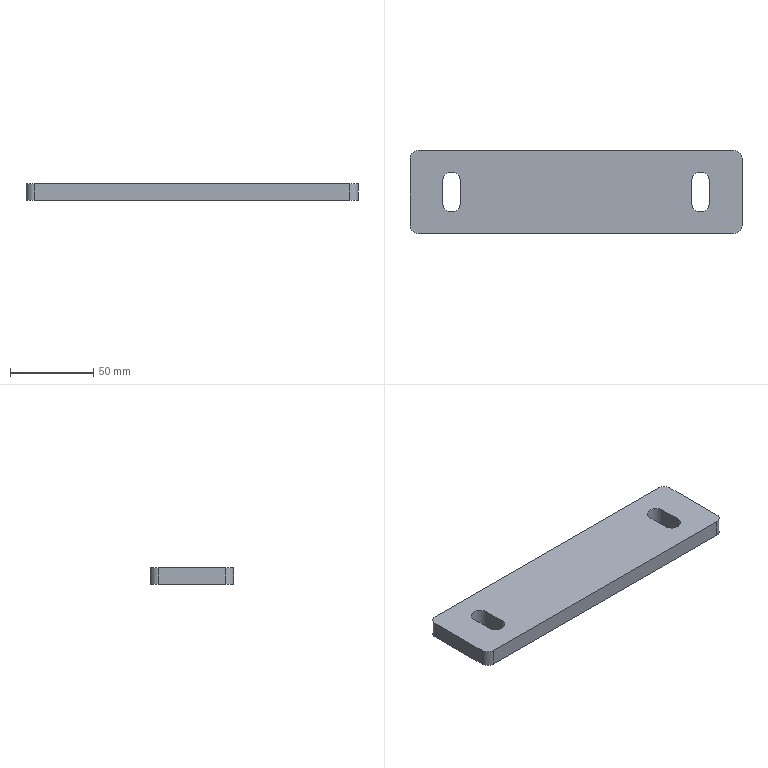Part | STEP file | 1 solid | 18 faces | box 200 x 50 x 10 mm | volume 95025 mm3 | plane 10 | cylinder 8 | commonest cylinder face diameters 10 x4 11 x4
STEP:
#1=CARTESIAN_POINT('',(0.,0.,0.));
#2=DIRECTION('',(0.,0.,1.));
#3=DIRECTION('',(1.,0.,0.));
#4=AXIS2_PLACEMENT_3D('',#1,#2,#3);
#5=CARTESIAN_POINT('',(-80.5,6.5,10.));
#6=VERTEX_POINT('',#5);
#7=CARTESIAN_POINT('',(-69.5,6.5,10.));
#8=VERTEX_POINT('',#7);
#9=CARTESIAN_POINT('',(-75.,6.5,10.));
#10=DIRECTION('',(0.,0.,-1.));
#11=DIRECTION('',(1.,0.,0.));
#12=AXIS2_PLACEMENT_3D('',#9,#10,#11);
#13=CIRCLE('',#12,5.5);
#14=CARTESIAN_POINT('',(95.,20.,10.));
#15=DIRECTION('',(0.,0.,1.));
#16=DIRECTION('',(1.,0.,0.));
#17=AXIS2_PLACEMENT_3D('',#14,#15,#16);
#18=PLANE('',#17);
#19=CARTESIAN_POINT('',(-164.5,-13.5));
#20=CARTESIAN_POINT('',(-164.5,-23.026));
#21=CARTESIAN_POINT('',(-172.75,-18.263));
#22=CARTESIAN_POINT('',(-181.,-13.5));
#23=CARTESIAN_POINT('',(-172.75,-8.737));
#24=CARTESIAN_POINT('',(-164.5,-3.974));
#25=CARTESIAN_POINT('',(-164.5,-13.5));
#26=(BOUNDED_CURVE()B_SPLINE_CURVE(2,(#19,#20,#21,#22,#23,#24,#25),.UNSPECIFIED.,.T.,.F.)B_SPLINE_CURVE_WITH_KNOTS((1,2,2,2,2,1),(-2.094,0.,2.094,4.189,6.283,8.378),.UNSPECIFIED.)CURVE()GEOMETRIC_REPRESENTATION_ITEM()RATIONAL_B_SPLINE_CURVE((1.,0.5,1.,0.5,1.,0.5,1.))REPRESENTATION_ITEM(''));
#27=(GEOMETRIC_REPRESENTATION_CONTEXT(2)PARAMETRIC_REPRESENTATION_CONTEXT()REPRESENTATION_CONTEXT('',''));
#28=DEFINITIONAL_REPRESENTATION('',(#26),#27);
#29=PCURVE('',#18,#28);
#30=CARTESIAN_POINT('',(-75.,6.5,0.));
#31=DIRECTION('',(0.,0.,1.));
#32=DIRECTION('',(1.,0.,0.));
#33=AXIS2_PLACEMENT_3D('',#30,#31,#32);
#34=CYLINDRICAL_SURFACE('',#33,5.5);
#35=CARTESIAN_POINT('',(6.283,10.));
#36=DIRECTION('',(-1.,0.));
#37=VECTOR('',#36,1.);
#38=LINE('',#35,#37);
#39=(GEOMETRIC_REPRESENTATION_CONTEXT(2)PARAMETRIC_REPRESENTATION_CONTEXT()REPRESENTATION_CONTEXT('',''));
#40=DEFINITIONAL_REPRESENTATION('',(#38),#39);
#41=PCURVE('',#34,#40);
#42=SURFACE_CURVE('',#13,(#29,#41),.PCURVE_S1.);
#43=EDGE_CURVE('',#6,#8,#42,.T.);
#44=ORIENTED_EDGE('',*,*,#43,.T.);
#45=CARTESIAN_POINT('',(-69.5,-6.5,10.));
#46=VERTEX_POINT('',#45);
#47=CARTESIAN_POINT('',(-69.5,-6.5,10.));
#48=DIRECTION('',(0.,-1.,0.));
#49=VECTOR('',#48,1.);
#50=LINE('',#47,#49);
#51=CARTESIAN_POINT('',(-164.5,-26.5));
#52=DIRECTION('',(0.,-1.));
#53=VECTOR('',#52,1.);
#54=LINE('',#51,#53);
#55=(GEOMETRIC_REPRESENTATION_CONTEXT(2)PARAMETRIC_REPRESENTATION_CONTEXT()REPRESENTATION_CONTEXT('',''));
#56=DEFINITIONAL_REPRESENTATION('',(#54),#55);
#57=PCURVE('',#18,#56);
#58=CARTESIAN_POINT('',(-69.5,-6.5,0.));
#59=DIRECTION('',(1.,0.,0.));
#60=DIRECTION('',(0.,1.,0.));
#61=AXIS2_PLACEMENT_3D('',#58,#59,#60);
#62=PLANE('',#61);
#63=CARTESIAN_POINT('',(0.,10.));
#64=DIRECTION('',(-1.,0.));
#65=VECTOR('',#64,1.);
#66=LINE('',#63,#65);
#67=(GEOMETRIC_REPRESENTATION_CONTEXT(2)PARAMETRIC_REPRESENTATION_CONTEXT()REPRESENTATION_CONTEXT('',''));
#68=DEFINITIONAL_REPRESENTATION('',(#66),#67);
#69=PCURVE('',#62,#68);
#70=SURFACE_CURVE('',#50,(#57,#69),.PCURVE_S1.);
#71=EDGE_CURVE('',#8,#46,#70,.T.);
#72=ORIENTED_EDGE('',*,*,#71,.T.);
#73=CARTESIAN_POINT('',(-80.5,-6.5,10.));
#74=VERTEX_POINT('',#73);
#75=CARTESIAN_POINT('',(-75.,-6.5,10.));
#76=DIRECTION('',(0.,0.,-1.));
#77=DIRECTION('',(1.,0.,0.));
#78=AXIS2_PLACEMENT_3D('',#75,#76,#77);
#79=CIRCLE('',#78,5.5);
#80=CARTESIAN_POINT('',(-164.5,-26.5));
#81=CARTESIAN_POINT('',(-164.5,-36.026));
#82=CARTESIAN_POINT('',(-172.75,-31.263));
#83=CARTESIAN_POINT('',(-181.,-26.5));
#84=CARTESIAN_POINT('',(-172.75,-21.737));
#85=CARTESIAN_POINT('',(-164.5,-16.974));
#86=CARTESIAN_POINT('',(-164.5,-26.5));
#87=(BOUNDED_CURVE()B_SPLINE_CURVE(2,(#80,#81,#82,#83,#84,#85,#86),.UNSPECIFIED.,.T.,.F.)B_SPLINE_CURVE_WITH_KNOTS((1,2,2,2,2,1),(-2.094,0.,2.094,4.189,6.283,8.378),.UNSPECIFIED.)CURVE()GEOMETRIC_REPRESENTATION_ITEM()RATIONAL_B_SPLINE_CURVE((1.,0.5,1.,0.5,1.,0.5,1.))REPRESENTATION_ITEM(''));
#88=(GEOMETRIC_REPRESENTATION_CONTEXT(2)PARAMETRIC_REPRESENTATION_CONTEXT()REPRESENTATION_CONTEXT('',''));
#89=DEFINITIONAL_REPRESENTATION('',(#87),#88);
#90=PCURVE('',#18,#89);
#91=CARTESIAN_POINT('',(-75.,-6.5,0.));
#92=DIRECTION('',(0.,0.,1.));
#93=DIRECTION('',(1.,0.,0.));
#94=AXIS2_PLACEMENT_3D('',#91,#92,#93);
#95=CYLINDRICAL_SURFACE('',#94,5.5);
#96=CARTESIAN_POINT('',(6.283,10.));
#97=DIRECTION('',(-1.,0.));
#98=VECTOR('',#97,1.);
#99=LINE('',#96,#98);
#100=(GEOMETRIC_REPRESENTATION_CONTEXT(2)PARAMETRIC_REPRESENTATION_CONTEXT()REPRESENTATION_CONTEXT('',''));
#101=DEFINITIONAL_REPRESENTATION('',(#99),#100);
#102=PCURVE('',#95,#101);
#103=SURFACE_CURVE('',#79,(#90,#102),.PCURVE_S1.);
#104=EDGE_CURVE('',#46,#74,#103,.T.);
#105=ORIENTED_EDGE('',*,*,#104,.T.);
#106=CARTESIAN_POINT('',(-80.5,-6.5,10.));
#107=DIRECTION('',(0.,1.,0.));
#108=VECTOR('',#107,1.);
#109=LINE('',#106,#108);
#110=CARTESIAN_POINT('',(-175.5,-26.5));
#111=DIRECTION('',(0.,1.));
#112=VECTOR('',#111,1.);
#113=LINE('',#110,#112);
#114=(GEOMETRIC_REPRESENTATION_CONTEXT(2)PARAMETRIC_REPRESENTATION_CONTEXT()REPRESENTATION_CONTEXT('',''));
#115=DEFINITIONAL_REPRESENTATION('',(#113),#114);
#116=PCURVE('',#18,#115);
#117=CARTESIAN_POINT('',(-80.5,-6.5,0.));
#118=DIRECTION('',(-1.,0.,0.));
#119=DIRECTION('',(0.,0.,1.));
#120=AXIS2_PLACEMENT_3D('',#117,#118,#119);
#121=PLANE('',#120);
#122=CARTESIAN_POINT('',(10.,0.));
#123=DIRECTION('',(0.,1.));
#124=VECTOR('',#123,1.);
#125=LINE('',#122,#124);
#126=(GEOMETRIC_REPRESENTATION_CONTEXT(2)PARAMETRIC_REPRESENTATION_CONTEXT()REPRESENTATION_CONTEXT('',''));
#127=DEFINITIONAL_REPRESENTATION('',(#125),#126);
#128=PCURVE('',#121,#127);
#129=SURFACE_CURVE('',#109,(#116,#128),.PCURVE_S1.);
#130=EDGE_CURVE('',#74,#6,#129,.T.);
#131=ORIENTED_EDGE('',*,*,#130,.T.);
#132=EDGE_LOOP('',(#44,#72,#105,#131));
#133=FACE_BOUND('',#132,.T.);
#134=CARTESIAN_POINT('',(69.5,6.5,10.));
#135=VERTEX_POINT('',#134);
#136=CARTESIAN_POINT('',(69.5,-6.5,10.));
#137=VERTEX_POINT('',#136);
#138=CARTESIAN_POINT('',(69.5,-6.5,10.));
#139=DIRECTION('',(0.,-1.,0.));
#140=VECTOR('',#139,1.);
#141=LINE('',#138,#140);
#142=CARTESIAN_POINT('',(-25.5,-26.5));
#143=DIRECTION('',(0.,-1.));
#144=VECTOR('',#143,1.);
#145=LINE('',#142,#144);
#146=(GEOMETRIC_REPRESENTATION_CONTEXT(2)PARAMETRIC_REPRESENTATION_CONTEXT()REPRESENTATION_CONTEXT('',''));
#147=DEFINITIONAL_REPRESENTATION('',(#145),#146);
#148=PCURVE('',#18,#147);
#149=CARTESIAN_POINT('',(69.5,-6.5,0.));
#150=DIRECTION('',(1.,0.,0.));
#151=DIRECTION('',(0.,1.,0.));
#152=AXIS2_PLACEMENT_3D('',#149,#150,#151);
#153=PLANE('',#152);
#154=CARTESIAN_POINT('',(0.,10.));
#155=DIRECTION('',(-1.,0.));
#156=VECTOR('',#155,1.);
#157=LINE('',#154,#156);
#158=(GEOMETRIC_REPRESENTATION_CONTEXT(2)PARAMETRIC_REPRESENTATION_CONTEXT()REPRESENTATION_CONTEXT('',''));
#159=DEFINITIONAL_REPRESENTATION('',(#157),#158);
#160=PCURVE('',#153,#159);
#161=SURFACE_CURVE('',#141,(#148,#160),.PCURVE_S1.);
#162=EDGE_CURVE('',#135,#137,#161,.T.);
#163=ORIENTED_EDGE('',*,*,#162,.F.);
#164=CARTESIAN_POINT('',(80.5,6.5,10.));
#165=VERTEX_POINT('',#164);
#166=CARTESIAN_POINT('',(75.,6.5,10.));
#167=DIRECTION('',(0.,0.,-1.));
#168=DIRECTION('',(1.,0.,0.));
#169=AXIS2_PLACEMENT_3D('',#166,#167,#168);
#170=CIRCLE('',#169,5.5);
#171=CARTESIAN_POINT('',(-14.5,-13.5));
#172=CARTESIAN_POINT('',(-14.5,-23.026));
#173=CARTESIAN_POINT('',(-22.75,-18.263));
#174=CARTESIAN_POINT('',(-31.,-13.5));
#175=CARTESIAN_POINT('',(-22.75,-8.737));
#176=CARTESIAN_POINT('',(-14.5,-3.974));
#177=CARTESIAN_POINT('',(-14.5,-13.5));
#178=(BOUNDED_CURVE()B_SPLINE_CURVE(2,(#171,#172,#173,#174,#175,#176,#177),.UNSPECIFIED.,.T.,.F.)B_SPLINE_CURVE_WITH_KNOTS((1,2,2,2,2,1),(-2.094,0.,2.094,4.189,6.283,8.378),.UNSPECIFIED.)CURVE()GEOMETRIC_REPRESENTATION_ITEM()RATIONAL_B_SPLINE_CURVE((1.,0.5,1.,0.5,1.,0.5,1.))REPRESENTATION_ITEM(''));
#179=(GEOMETRIC_REPRESENTATION_CONTEXT(2)PARAMETRIC_REPRESENTATION_CONTEXT()REPRESENTATION_CONTEXT('',''));
#180=DEFINITIONAL_REPRESENTATION('',(#178),#179);
#181=PCURVE('',#18,#180);
#182=CARTESIAN_POINT('',(75.,6.5,0.));
#183=DIRECTION('',(0.,0.,1.));
#184=DIRECTION('',(1.,0.,0.));
#185=AXIS2_PLACEMENT_3D('',#182,#183,#184);
#186=CYLINDRICAL_SURFACE('',#185,5.5);
#187=CARTESIAN_POINT('',(6.283,10.));
#188=DIRECTION('',(-1.,0.));
#189=VECTOR('',#188,1.);
#190=LINE('',#187,#189);
#191=(GEOMETRIC_REPRESENTATION_CONTEXT(2)PARAMETRIC_REPRESENTATION_CONTEXT()REPRESENTATION_CONTEXT('',''));
#192=DEFINITIONAL_REPRESENTATION('',(#190),#191);
#193=PCURVE('',#186,#192);
#194=SURFACE_CURVE('',#170,(#181,#193),.PCURVE_S1.);
#195=EDGE_CURVE('',#135,#165,#194,.T.);
#196=ORIENTED_EDGE('',*,*,#195,.T.);
#197=CARTESIAN_POINT('',(80.5,-6.5,10.));
#198=VERTEX_POINT('',#197);
#199=CARTESIAN_POINT('',(80.5,-6.5,10.));
#200=DIRECTION('',(0.,1.,0.));
#201=VECTOR('',#200,1.);
#202=LINE('',#199,#201);
#203=CARTESIAN_POINT('',(-14.5,-26.5));
#204=DIRECTION('',(0.,1.));
#205=VECTOR('',#204,1.);
#206=LINE('',#203,#205);
#207=(GEOMETRIC_REPRESENTATION_CONTEXT(2)PARAMETRIC_REPRESENTATION_CONTEXT()REPRESENTATION_CONTEXT('',''));
#208=DEFINITIONAL_REPRESENTATION('',(#206),#207);
#209=PCURVE('',#18,#208);
#210=CARTESIAN_POINT('',(80.5,-6.5,0.));
#211=DIRECTION('',(-1.,0.,0.));
#212=DIRECTION('',(0.,0.,1.));
#213=AXIS2_PLACEMENT_3D('',#210,#211,#212);
#214=PLANE('',#213);
#215=CARTESIAN_POINT('',(10.,0.));
#216=DIRECTION('',(0.,1.));
#217=VECTOR('',#216,1.);
#218=LINE('',#215,#217);
#219=(GEOMETRIC_REPRESENTATION_CONTEXT(2)PARAMETRIC_REPRESENTATION_CONTEXT()REPRESENTATION_CONTEXT('',''));
#220=DEFINITIONAL_REPRESENTATION('',(#218),#219);
#221=PCURVE('',#214,#220);
#222=SURFACE_CURVE('',#202,(#209,#221),.PCURVE_S1.);
#223=EDGE_CURVE('',#198,#165,#222,.T.);
#224=ORIENTED_EDGE('',*,*,#223,.F.);
#225=CARTESIAN_POINT('',(75.,-6.5,10.));
#226=DIRECTION('',(0.,0.,-1.));
#227=DIRECTION('',(1.,0.,0.));
#228=AXIS2_PLACEMENT_3D('',#225,#226,#227);
#229=CIRCLE('',#228,5.5);
#230=CARTESIAN_POINT('',(-14.5,-26.5));
#231=CARTESIAN_POINT('',(-14.5,-36.026));
#232=CARTESIAN_POINT('',(-22.75,-31.263));
#233=CARTESIAN_POINT('',(-31.,-26.5));
#234=CARTESIAN_POINT('',(-22.75,-21.737));
#235=CARTESIAN_POINT('',(-14.5,-16.974));
#236=CARTESIAN_POINT('',(-14.5,-26.5));
#237=(BOUNDED_CURVE()B_SPLINE_CURVE(2,(#230,#231,#232,#233,#234,#235,#236),.UNSPECIFIED.,.T.,.F.)B_SPLINE_CURVE_WITH_KNOTS((1,2,2,2,2,1),(-2.094,0.,2.094,4.189,6.283,8.378),.UNSPECIFIED.)CURVE()GEOMETRIC_REPRESENTATION_ITEM()RATIONAL_B_SPLINE_CURVE((1.,0.5,1.,0.5,1.,0.5,1.))REPRESENTATION_ITEM(''));
#238=(GEOMETRIC_REPRESENTATION_CONTEXT(2)PARAMETRIC_REPRESENTATION_CONTEXT()REPRESENTATION_CONTEXT('',''));
#239=DEFINITIONAL_REPRESENTATION('',(#237),#238);
#240=PCURVE('',#18,#239);
#241=CARTESIAN_POINT('',(75.,-6.5,0.));
#242=DIRECTION('',(0.,0.,1.));
#243=DIRECTION('',(1.,0.,0.));
#244=AXIS2_PLACEMENT_3D('',#241,#242,#243);
#245=CYLINDRICAL_SURFACE('',#244,5.5);
#246=CARTESIAN_POINT('',(6.283,10.));
#247=DIRECTION('',(-1.,0.));
#248=VECTOR('',#247,1.);
#249=LINE('',#246,#248);
#250=(GEOMETRIC_REPRESENTATION_CONTEXT(2)PARAMETRIC_REPRESENTATION_CONTEXT()REPRESENTATION_CONTEXT('',''));
#251=DEFINITIONAL_REPRESENTATION('',(#249),#250);
#252=PCURVE('',#245,#251);
#253=SURFACE_CURVE('',#229,(#240,#252),.PCURVE_S1.);
#254=EDGE_CURVE('',#198,#137,#253,.T.);
#255=ORIENTED_EDGE('',*,*,#254,.T.);
#256=EDGE_LOOP('',(#163,#196,#224,#255));
#257=FACE_BOUND('',#256,.T.);
#258=CARTESIAN_POINT('',(100.,-20.,10.));
#259=VERTEX_POINT('',#258);
#260=CARTESIAN_POINT('',(95.,-25.,10.));
#261=VERTEX_POINT('',#260);
#262=CARTESIAN_POINT('',(95.,-20.,10.));
#263=DIRECTION('',(0.,0.,-1.));
#264=DIRECTION('',(-1.,0.,0.));
#265=AXIS2_PLACEMENT_3D('',#262,#263,#264);
#266=CIRCLE('',#265,5.);
#267=CARTESIAN_POINT('',(-5.,-40.));
#268=CARTESIAN_POINT('',(-5.,-31.34));
#269=CARTESIAN_POINT('',(2.5,-35.67));
#270=CARTESIAN_POINT('',(10.,-40.));
#271=CARTESIAN_POINT('',(2.5,-44.33));
#272=CARTESIAN_POINT('',(-5.,-48.66));
#273=CARTESIAN_POINT('',(-5.,-40.));
#274=(BOUNDED_CURVE()B_SPLINE_CURVE(2,(#267,#268,#269,#270,#271,#272,#273),.UNSPECIFIED.,.T.,.F.)B_SPLINE_CURVE_WITH_KNOTS((1,2,2,2,2,1),(-2.094,0.,2.094,4.189,6.283,8.378),.UNSPECIFIED.)CURVE()GEOMETRIC_REPRESENTATION_ITEM()RATIONAL_B_SPLINE_CURVE((1.,0.5,1.,0.5,1.,0.5,1.))REPRESENTATION_ITEM(''));
#275=(GEOMETRIC_REPRESENTATION_CONTEXT(2)PARAMETRIC_REPRESENTATION_CONTEXT()REPRESENTATION_CONTEXT('',''));
#276=DEFINITIONAL_REPRESENTATION('',(#274),#275);
#277=PCURVE('',#18,#276);
#278=CARTESIAN_POINT('',(95.,-20.,10.));
#279=DIRECTION('',(0.,0.,-1.));
#280=DIRECTION('',(-1.,0.,0.));
#281=AXIS2_PLACEMENT_3D('',#278,#279,#280);
#282=CYLINDRICAL_SURFACE('',#281,5.);
#283=CARTESIAN_POINT('',(0.,0.));
#284=DIRECTION('',(1.,0.));
#285=VECTOR('',#284,1.);
#286=LINE('',#283,#285);
#287=(GEOMETRIC_REPRESENTATION_CONTEXT(2)PARAMETRIC_REPRESENTATION_CONTEXT()REPRESENTATION_CONTEXT('',''));
#288=DEFINITIONAL_REPRESENTATION('',(#286),#287);
#289=PCURVE('',#282,#288);
#290=SURFACE_CURVE('',#266,(#277,#289),.PCURVE_S1.);
#291=EDGE_CURVE('',#259,#261,#290,.T.);
#292=ORIENTED_EDGE('',*,*,#291,.F.);
#293=CARTESIAN_POINT('',(100.,20.,10.));
#294=VERTEX_POINT('',#293);
#295=CARTESIAN_POINT('',(100.,-20.,10.));
#296=DIRECTION('',(0.,1.,0.));
#297=VECTOR('',#296,1.);
#298=LINE('',#295,#297);
#299=CARTESIAN_POINT('',(5.,-40.));
#300=DIRECTION('',(0.,1.));
#301=VECTOR('',#300,1.);
#302=LINE('',#299,#301);
#303=(GEOMETRIC_REPRESENTATION_CONTEXT(2)PARAMETRIC_REPRESENTATION_CONTEXT()REPRESENTATION_CONTEXT('',''));
#304=DEFINITIONAL_REPRESENTATION('',(#302),#303);
#305=PCURVE('',#18,#304);
#306=CARTESIAN_POINT('',(100.,-20.,10.));
#307=DIRECTION('',(-1.,0.,0.));
#308=DIRECTION('',(0.,0.,1.));
#309=AXIS2_PLACEMENT_3D('',#306,#307,#308);
#310=PLANE('',#309);
#311=CARTESIAN_POINT('',(0.,0.));
#312=DIRECTION('',(0.,1.));
#313=VECTOR('',#312,1.);
#314=LINE('',#311,#313);
#315=(GEOMETRIC_REPRESENTATION_CONTEXT(2)PARAMETRIC_REPRESENTATION_CONTEXT()REPRESENTATION_CONTEXT('',''));
#316=DEFINITIONAL_REPRESENTATION('',(#314),#315);
#317=PCURVE('',#310,#316);
#318=SURFACE_CURVE('',#298,(#305,#317),.PCURVE_S1.);
#319=EDGE_CURVE('',#259,#294,#318,.T.);
#320=ORIENTED_EDGE('',*,*,#319,.T.);
#321=CARTESIAN_POINT('',(95.,25.,10.));
#322=VERTEX_POINT('',#321);
#323=CARTESIAN_POINT('',(95.,20.,10.));
#324=DIRECTION('',(0.,0.,-1.));
#325=DIRECTION('',(-1.,0.,0.));
#326=AXIS2_PLACEMENT_3D('',#323,#324,#325);
#327=CIRCLE('',#326,5.);
#328=CARTESIAN_POINT('',(-5.,0.));
#329=CARTESIAN_POINT('',(-5.,8.66));
#330=CARTESIAN_POINT('',(2.5,4.33));
#331=CARTESIAN_POINT('',(10.,0.));
#332=CARTESIAN_POINT('',(2.5,-4.33));
#333=CARTESIAN_POINT('',(-5.,-8.66));
#334=CARTESIAN_POINT('',(-5.,0.));
#335=(BOUNDED_CURVE()B_SPLINE_CURVE(2,(#328,#329,#330,#331,#332,#333,#334),.UNSPECIFIED.,.T.,.F.)B_SPLINE_CURVE_WITH_KNOTS((1,2,2,2,2,1),(-2.094,0.,2.094,4.189,6.283,8.378),.UNSPECIFIED.)CURVE()GEOMETRIC_REPRESENTATION_ITEM()RATIONAL_B_SPLINE_CURVE((1.,0.5,1.,0.5,1.,0.5,1.))REPRESENTATION_ITEM(''));
#336=(GEOMETRIC_REPRESENTATION_CONTEXT(2)PARAMETRIC_REPRESENTATION_CONTEXT()REPRESENTATION_CONTEXT('',''));
#337=DEFINITIONAL_REPRESENTATION('',(#335),#336);
#338=PCURVE('',#18,#337);
#339=CARTESIAN_POINT('',(95.,20.,10.));
#340=DIRECTION('',(0.,0.,-1.));
#341=DIRECTION('',(-1.,0.,0.));
#342=AXIS2_PLACEMENT_3D('',#339,#340,#341);
#343=CYLINDRICAL_SURFACE('',#342,5.);
#344=CARTESIAN_POINT('',(0.,0.));
#345=DIRECTION('',(1.,0.));
#346=VECTOR('',#345,1.);
#347=LINE('',#344,#346);
#348=(GEOMETRIC_REPRESENTATION_CONTEXT(2)PARAMETRIC_REPRESENTATION_CONTEXT()REPRESENTATION_CONTEXT('',''));
#349=DEFINITIONAL_REPRESENTATION('',(#347),#348);
#350=PCURVE('',#343,#349);
#351=SURFACE_CURVE('',#327,(#338,#350),.PCURVE_S1.);
#352=EDGE_CURVE('',#322,#294,#351,.T.);
#353=ORIENTED_EDGE('',*,*,#352,.F.);
#354=CARTESIAN_POINT('',(-95.,25.,10.));
#355=VERTEX_POINT('',#354);
#356=CARTESIAN_POINT('',(95.,25.,10.));
#357=DIRECTION('',(-1.,0.,0.));
#358=VECTOR('',#357,1.);
#359=LINE('',#356,#358);
#360=CARTESIAN_POINT('',(0.,5.));
#361=DIRECTION('',(-1.,0.));
#362=VECTOR('',#361,1.);
#363=LINE('',#360,#362);
#364=(GEOMETRIC_REPRESENTATION_CONTEXT(2)PARAMETRIC_REPRESENTATION_CONTEXT()REPRESENTATION_CONTEXT('',''));
#365=DEFINITIONAL_REPRESENTATION('',(#363),#364);
#366=PCURVE('',#18,#365);
#367=CARTESIAN_POINT('',(95.,25.,10.));
#368=DIRECTION('',(0.,-1.,0.));
#369=DIRECTION('',(0.,0.,-1.));
#370=AXIS2_PLACEMENT_3D('',#367,#368,#369);
#371=PLANE('',#370);
#372=CARTESIAN_POINT('',(0.,0.));
#373=DIRECTION('',(0.,-1.));
#374=VECTOR('',#373,1.);
#375=LINE('',#372,#374);
#376=(GEOMETRIC_REPRESENTATION_CONTEXT(2)PARAMETRIC_REPRESENTATION_CONTEXT()REPRESENTATION_CONTEXT('',''));
#377=DEFINITIONAL_REPRESENTATION('',(#375),#376);
#378=PCURVE('',#371,#377);
#379=SURFACE_CURVE('',#359,(#366,#378),.PCURVE_S1.);
#380=EDGE_CURVE('',#322,#355,#379,.T.);
#381=ORIENTED_EDGE('',*,*,#380,.T.);
#382=CARTESIAN_POINT('',(-100.,20.,10.));
#383=VERTEX_POINT('',#382);
#384=CARTESIAN_POINT('',(-95.,20.,10.));
#385=DIRECTION('',(0.,0.,-1.));
#386=DIRECTION('',(-1.,0.,0.));
#387=AXIS2_PLACEMENT_3D('',#384,#385,#386);
#388=CIRCLE('',#387,5.);
#389=CARTESIAN_POINT('',(-195.,0.));
#390=CARTESIAN_POINT('',(-195.,8.66));
#391=CARTESIAN_POINT('',(-187.5,4.33));
#392=CARTESIAN_POINT('',(-180.,0.));
#393=CARTESIAN_POINT('',(-187.5,-4.33));
#394=CARTESIAN_POINT('',(-195.,-8.66));
#395=CARTESIAN_POINT('',(-195.,0.));
#396=(BOUNDED_CURVE()B_SPLINE_CURVE(2,(#389,#390,#391,#392,#393,#394,#395),.UNSPECIFIED.,.T.,.F.)B_SPLINE_CURVE_WITH_KNOTS((1,2,2,2,2,1),(-2.094,0.,2.094,4.189,6.283,8.378),.UNSPECIFIED.)CURVE()GEOMETRIC_REPRESENTATION_ITEM()RATIONAL_B_SPLINE_CURVE((1.,0.5,1.,0.5,1.,0.5,1.))REPRESENTATION_ITEM(''));
#397=(GEOMETRIC_REPRESENTATION_CONTEXT(2)PARAMETRIC_REPRESENTATION_CONTEXT()REPRESENTATION_CONTEXT('',''));
#398=DEFINITIONAL_REPRESENTATION('',(#396),#397);
#399=PCURVE('',#18,#398);
#400=CARTESIAN_POINT('',(-95.,20.,10.));
#401=DIRECTION('',(0.,0.,-1.));
#402=DIRECTION('',(-1.,0.,0.));
#403=AXIS2_PLACEMENT_3D('',#400,#401,#402);
#404=CYLINDRICAL_SURFACE('',#403,5.);
#405=CARTESIAN_POINT('',(0.,0.));
#406=DIRECTION('',(1.,0.));
#407=VECTOR('',#406,1.);
#408=LINE('',#405,#407);
#409=(GEOMETRIC_REPRESENTATION_CONTEXT(2)PARAMETRIC_REPRESENTATION_CONTEXT()REPRESENTATION_CONTEXT('',''));
#410=DEFINITIONAL_REPRESENTATION('',(#408),#409);
#411=PCURVE('',#404,#410);
#412=SURFACE_CURVE('',#388,(#399,#411),.PCURVE_S1.);
#413=EDGE_CURVE('',#383,#355,#412,.T.);
#414=ORIENTED_EDGE('',*,*,#413,.F.);
#415=CARTESIAN_POINT('',(-100.,-20.,10.));
#416=VERTEX_POINT('',#415);
#417=CARTESIAN_POINT('',(-100.,-20.,10.));
#418=DIRECTION('',(0.,1.,0.));
#419=VECTOR('',#418,1.);
#420=LINE('',#417,#419);
#421=CARTESIAN_POINT('',(-195.,-40.));
#422=DIRECTION('',(0.,1.));
#423=VECTOR('',#422,1.);
#424=LINE('',#421,#423);
#425=(GEOMETRIC_REPRESENTATION_CONTEXT(2)PARAMETRIC_REPRESENTATION_CONTEXT()REPRESENTATION_CONTEXT('',''));
#426=DEFINITIONAL_REPRESENTATION('',(#424),#425);
#427=PCURVE('',#18,#426);
#428=CARTESIAN_POINT('',(-100.,-20.,10.));
#429=DIRECTION('',(-1.,0.,0.));
#430=DIRECTION('',(0.,0.,1.));
#431=AXIS2_PLACEMENT_3D('',#428,#429,#430);
#432=PLANE('',#431);
#433=CARTESIAN_POINT('',(0.,0.));
#434=DIRECTION('',(0.,1.));
#435=VECTOR('',#434,1.);
#436=LINE('',#433,#435);
#437=(GEOMETRIC_REPRESENTATION_CONTEXT(2)PARAMETRIC_REPRESENTATION_CONTEXT()REPRESENTATION_CONTEXT('',''));
#438=DEFINITIONAL_REPRESENTATION('',(#436),#437);
#439=PCURVE('',#432,#438);
#440=SURFACE_CURVE('',#420,(#427,#439),.PCURVE_S1.);
#441=EDGE_CURVE('',#416,#383,#440,.T.);
#442=ORIENTED_EDGE('',*,*,#441,.F.);
#443=CARTESIAN_POINT('',(-95.,-25.,10.));
#444=VERTEX_POINT('',#443);
#445=CARTESIAN_POINT('',(-95.,-20.,10.));
#446=DIRECTION('',(0.,0.,-1.));
#447=DIRECTION('',(-1.,0.,0.));
#448=AXIS2_PLACEMENT_3D('',#445,#446,#447);
#449=CIRCLE('',#448,5.);
#450=CARTESIAN_POINT('',(-195.,-40.));
#451=CARTESIAN_POINT('',(-195.,-31.34));
#452=CARTESIAN_POINT('',(-187.5,-35.67));
#453=CARTESIAN_POINT('',(-180.,-40.));
#454=CARTESIAN_POINT('',(-187.5,-44.33));
#455=CARTESIAN_POINT('',(-195.,-48.66));
#456=CARTESIAN_POINT('',(-195.,-40.));
#457=(BOUNDED_CURVE()B_SPLINE_CURVE(2,(#450,#451,#452,#453,#454,#455,#456),.UNSPECIFIED.,.T.,.F.)B_SPLINE_CURVE_WITH_KNOTS((1,2,2,2,2,1),(-2.094,0.,2.094,4.189,6.283,8.378),.UNSPECIFIED.)CURVE()GEOMETRIC_REPRESENTATION_ITEM()RATIONAL_B_SPLINE_CURVE((1.,0.5,1.,0.5,1.,0.5,1.))REPRESENTATION_ITEM(''));
#458=(GEOMETRIC_REPRESENTATION_CONTEXT(2)PARAMETRIC_REPRESENTATION_CONTEXT()REPRESENTATION_CONTEXT('',''));
#459=DEFINITIONAL_REPRESENTATION('',(#457),#458);
#460=PCURVE('',#18,#459);
#461=CARTESIAN_POINT('',(-95.,-20.,10.));
#462=DIRECTION('',(0.,0.,-1.));
#463=DIRECTION('',(-1.,0.,0.));
#464=AXIS2_PLACEMENT_3D('',#461,#462,#463);
#465=CYLINDRICAL_SURFACE('',#464,5.);
#466=CARTESIAN_POINT('',(0.,0.));
#467=DIRECTION('',(1.,0.));
#468=VECTOR('',#467,1.);
#469=LINE('',#466,#468);
#470=(GEOMETRIC_REPRESENTATION_CONTEXT(2)PARAMETRIC_REPRESENTATION_CONTEXT()REPRESENTATION_CONTEXT('',''));
#471=DEFINITIONAL_REPRESENTATION('',(#469),#470);
#472=PCURVE('',#465,#471);
#473=SURFACE_CURVE('',#449,(#460,#472),.PCURVE_S1.);
#474=EDGE_CURVE('',#444,#416,#473,.T.);
#475=ORIENTED_EDGE('',*,*,#474,.F.);
#476=CARTESIAN_POINT('',(95.,-25.,10.));
#477=DIRECTION('',(-1.,0.,0.));
#478=VECTOR('',#477,1.);
#479=LINE('',#476,#478);
#480=CARTESIAN_POINT('',(0.,-45.));
#481=DIRECTION('',(-1.,0.));
#482=VECTOR('',#481,1.);
#483=LINE('',#480,#482);
#484=(GEOMETRIC_REPRESENTATION_CONTEXT(2)PARAMETRIC_REPRESENTATION_CONTEXT()REPRESENTATION_CONTEXT('',''));
#485=DEFINITIONAL_REPRESENTATION('',(#483),#484);
#486=PCURVE('',#18,#485);
#487=CARTESIAN_POINT('',(95.,-25.,10.));
#488=DIRECTION('',(0.,-1.,0.));
#489=DIRECTION('',(0.,0.,-1.));
#490=AXIS2_PLACEMENT_3D('',#487,#488,#489);
#491=PLANE('',#490);
#492=CARTESIAN_POINT('',(0.,0.));
#493=DIRECTION('',(0.,-1.));
#494=VECTOR('',#493,1.);
#495=LINE('',#492,#494);
#496=(GEOMETRIC_REPRESENTATION_CONTEXT(2)PARAMETRIC_REPRESENTATION_CONTEXT()REPRESENTATION_CONTEXT('',''));
#497=DEFINITIONAL_REPRESENTATION('',(#495),#496);
#498=PCURVE('',#491,#497);
#499=SURFACE_CURVE('',#479,(#486,#498),.PCURVE_S1.);
#500=EDGE_CURVE('',#261,#444,#499,.T.);
#501=ORIENTED_EDGE('',*,*,#500,.F.);
#502=EDGE_LOOP('',(#292,#320,#353,#381,#414,#442,#475,#501));
#503=FACE_BOUND('',#502,.T.);
#504=ADVANCED_FACE('',(#133,#257,#503),#18,.T.);
#505=CARTESIAN_POINT('',(-95.,25.,0.));
#506=VERTEX_POINT('',#505);
#507=CARTESIAN_POINT('',(-95.,25.,10.));
#508=DIRECTION('',(0.,0.,-1.));
#509=VECTOR('',#508,1.);
#510=LINE('',#507,#509);
#511=CARTESIAN_POINT('',(0.,-190.));
#512=DIRECTION('',(1.,0.));
#513=VECTOR('',#512,1.);
#514=LINE('',#511,#513);
#515=(GEOMETRIC_REPRESENTATION_CONTEXT(2)PARAMETRIC_REPRESENTATION_CONTEXT()REPRESENTATION_CONTEXT('',''));
#516=DEFINITIONAL_REPRESENTATION('',(#514),#515);
#517=PCURVE('',#371,#516);
#518=CARTESIAN_POINT('',(1.571,0.));
#519=DIRECTION('',(0.,1.));
#520=VECTOR('',#519,1.);
#521=LINE('',#518,#520);
#522=(GEOMETRIC_REPRESENTATION_CONTEXT(2)PARAMETRIC_REPRESENTATION_CONTEXT()REPRESENTATION_CONTEXT('',''));
#523=DEFINITIONAL_REPRESENTATION('',(#521),#522);
#524=PCURVE('',#404,#523);
#525=SURFACE_CURVE('',#510,(#517,#524),.PCURVE_S1.);
#526=EDGE_CURVE('',#355,#506,#525,.T.);
#527=ORIENTED_EDGE('',*,*,#526,.F.);
#528=ORIENTED_EDGE('',*,*,#380,.F.);
#529=CARTESIAN_POINT('',(95.,25.,0.));
#530=VERTEX_POINT('',#529);
#531=CARTESIAN_POINT('',(95.,25.,10.));
#532=DIRECTION('',(0.,0.,1.));
#533=VECTOR('',#532,1.);
#534=LINE('',#531,#533);
#535=CARTESIAN_POINT('',(0.,0.));
#536=DIRECTION('',(-1.,0.));
#537=VECTOR('',#536,1.);
#538=LINE('',#535,#537);
#539=(GEOMETRIC_REPRESENTATION_CONTEXT(2)PARAMETRIC_REPRESENTATION_CONTEXT()REPRESENTATION_CONTEXT('',''));
#540=DEFINITIONAL_REPRESENTATION('',(#538),#539);
#541=PCURVE('',#371,#540);
#542=CARTESIAN_POINT('',(1.571,0.));
#543=DIRECTION('',(0.,-1.));
#544=VECTOR('',#543,1.);
#545=LINE('',#542,#544);
#546=(GEOMETRIC_REPRESENTATION_CONTEXT(2)PARAMETRIC_REPRESENTATION_CONTEXT()REPRESENTATION_CONTEXT('',''));
#547=DEFINITIONAL_REPRESENTATION('',(#545),#546);
#548=PCURVE('',#343,#547);
#549=SURFACE_CURVE('',#534,(#541,#548),.PCURVE_S1.);
#550=EDGE_CURVE('',#530,#322,#549,.T.);
#551=ORIENTED_EDGE('',*,*,#550,.F.);
#552=CARTESIAN_POINT('',(95.,25.,0.));
#553=DIRECTION('',(-1.,0.,0.));
#554=VECTOR('',#553,1.);
#555=LINE('',#552,#554);
#556=CARTESIAN_POINT('',(10.,0.));
#557=DIRECTION('',(0.,-1.));
#558=VECTOR('',#557,1.);
#559=LINE('',#556,#558);
#560=(GEOMETRIC_REPRESENTATION_CONTEXT(2)PARAMETRIC_REPRESENTATION_CONTEXT()REPRESENTATION_CONTEXT('',''));
#561=DEFINITIONAL_REPRESENTATION('',(#559),#560);
#562=PCURVE('',#371,#561);
#563=CARTESIAN_POINT('',(95.,20.,0.));
#564=DIRECTION('',(0.,0.,1.));
#565=DIRECTION('',(1.,0.,0.));
#566=AXIS2_PLACEMENT_3D('',#563,#564,#565);
#567=PLANE('',#566);
#568=CARTESIAN_POINT('',(0.,5.));
#569=DIRECTION('',(-1.,0.));
#570=VECTOR('',#569,1.);
#571=LINE('',#568,#570);
#572=(GEOMETRIC_REPRESENTATION_CONTEXT(2)PARAMETRIC_REPRESENTATION_CONTEXT()REPRESENTATION_CONTEXT('',''));
#573=DEFINITIONAL_REPRESENTATION('',(#571),#572);
#574=PCURVE('',#567,#573);
#575=SURFACE_CURVE('',#555,(#562,#574),.PCURVE_S1.);
#576=EDGE_CURVE('',#530,#506,#575,.T.);
#577=ORIENTED_EDGE('',*,*,#576,.T.);
#578=EDGE_LOOP('',(#527,#528,#551,#577));
#579=FACE_BOUND('',#578,.T.);
#580=ADVANCED_FACE('',(#579),#371,.F.);
#581=ORIENTED_EDGE('',*,*,#413,.T.);
#582=ORIENTED_EDGE('',*,*,#526,.T.);
#583=CARTESIAN_POINT('',(-100.,20.,0.));
#584=VERTEX_POINT('',#583);
#585=CARTESIAN_POINT('',(-95.,20.,0.));
#586=DIRECTION('',(0.,0.,1.));
#587=DIRECTION('',(-1.,0.,0.));
#588=AXIS2_PLACEMENT_3D('',#585,#586,#587);
#589=CIRCLE('',#588,5.);
#590=CARTESIAN_POINT('',(6.283,10.));
#591=DIRECTION('',(-1.,0.));
#592=VECTOR('',#591,1.);
#593=LINE('',#590,#592);
#594=(GEOMETRIC_REPRESENTATION_CONTEXT(2)PARAMETRIC_REPRESENTATION_CONTEXT()REPRESENTATION_CONTEXT('',''));
#595=DEFINITIONAL_REPRESENTATION('',(#593),#594);
#596=PCURVE('',#404,#595);
#597=CARTESIAN_POINT('',(-190.,0.));
#598=DIRECTION('',(-1.,0.));
#599=AXIS2_PLACEMENT_2D('',#597,#598);
#600=CIRCLE('',#599,5.);
#601=(GEOMETRIC_REPRESENTATION_CONTEXT(2)PARAMETRIC_REPRESENTATION_CONTEXT()REPRESENTATION_CONTEXT('',''));
#602=DEFINITIONAL_REPRESENTATION('',(#600),#601);
#603=PCURVE('',#567,#602);
#604=SURFACE_CURVE('',#589,(#596,#603),.PCURVE_S1.);
#605=EDGE_CURVE('',#506,#584,#604,.T.);
#606=ORIENTED_EDGE('',*,*,#605,.T.);
#607=CARTESIAN_POINT('',(-100.,20.,10.));
#608=DIRECTION('',(0.,0.,-1.));
#609=VECTOR('',#608,1.);
#610=LINE('',#607,#609);
#611=CARTESIAN_POINT('',(0.,0.));
#612=DIRECTION('',(0.,1.));
#613=VECTOR('',#612,1.);
#614=LINE('',#611,#613);
#615=(GEOMETRIC_REPRESENTATION_CONTEXT(2)PARAMETRIC_REPRESENTATION_CONTEXT()REPRESENTATION_CONTEXT('',''));
#616=DEFINITIONAL_REPRESENTATION('',(#614),#615);
#617=PCURVE('',#404,#616);
#618=CARTESIAN_POINT('',(0.,40.));
#619=DIRECTION('',(-1.,0.));
#620=VECTOR('',#619,1.);
#621=LINE('',#618,#620);
#622=(GEOMETRIC_REPRESENTATION_CONTEXT(2)PARAMETRIC_REPRESENTATION_CONTEXT()REPRESENTATION_CONTEXT('',''));
#623=DEFINITIONAL_REPRESENTATION('',(#621),#622);
#624=PCURVE('',#432,#623);
#625=SURFACE_CURVE('',#610,(#617,#624),.PCURVE_S1.);
#626=EDGE_CURVE('',#383,#584,#625,.T.);
#627=ORIENTED_EDGE('',*,*,#626,.F.);
#628=EDGE_LOOP('',(#581,#582,#606,#627));
#629=FACE_BOUND('',#628,.T.);
#630=ADVANCED_FACE('',(#629),#404,.T.);
#631=ORIENTED_EDGE('',*,*,#441,.T.);
#632=ORIENTED_EDGE('',*,*,#626,.T.);
#633=CARTESIAN_POINT('',(-100.,-20.,0.));
#634=VERTEX_POINT('',#633);
#635=CARTESIAN_POINT('',(-100.,20.,0.));
#636=DIRECTION('',(0.,-1.,0.));
#637=VECTOR('',#636,1.);
#638=LINE('',#635,#637);
#639=CARTESIAN_POINT('',(-10.,40.));
#640=DIRECTION('',(0.,-1.));
#641=VECTOR('',#640,1.);
#642=LINE('',#639,#641);
#643=(GEOMETRIC_REPRESENTATION_CONTEXT(2)PARAMETRIC_REPRESENTATION_CONTEXT()REPRESENTATION_CONTEXT('',''));
#644=DEFINITIONAL_REPRESENTATION('',(#642),#643);
#645=PCURVE('',#432,#644);
#646=CARTESIAN_POINT('',(-195.,0.));
#647=DIRECTION('',(0.,-1.));
#648=VECTOR('',#647,1.);
#649=LINE('',#646,#648);
#650=(GEOMETRIC_REPRESENTATION_CONTEXT(2)PARAMETRIC_REPRESENTATION_CONTEXT()REPRESENTATION_CONTEXT('',''));
#651=DEFINITIONAL_REPRESENTATION('',(#649),#650);
#652=PCURVE('',#567,#651);
#653=SURFACE_CURVE('',#638,(#645,#652),.PCURVE_S1.);
#654=EDGE_CURVE('',#584,#634,#653,.T.);
#655=ORIENTED_EDGE('',*,*,#654,.T.);
#656=CARTESIAN_POINT('',(-100.,-20.,10.));
#657=DIRECTION('',(0.,0.,-1.));
#658=VECTOR('',#657,1.);
#659=LINE('',#656,#658);
#660=CARTESIAN_POINT('',(0.,0.));
#661=DIRECTION('',(-1.,0.));
#662=VECTOR('',#661,1.);
#663=LINE('',#660,#662);
#664=(GEOMETRIC_REPRESENTATION_CONTEXT(2)PARAMETRIC_REPRESENTATION_CONTEXT()REPRESENTATION_CONTEXT('',''));
#665=DEFINITIONAL_REPRESENTATION('',(#663),#664);
#666=PCURVE('',#432,#665);
#667=CARTESIAN_POINT('',(6.283,0.));
#668=DIRECTION('',(0.,1.));
#669=VECTOR('',#668,1.);
#670=LINE('',#667,#669);
#671=(GEOMETRIC_REPRESENTATION_CONTEXT(2)PARAMETRIC_REPRESENTATION_CONTEXT()REPRESENTATION_CONTEXT('',''));
#672=DEFINITIONAL_REPRESENTATION('',(#670),#671);
#673=PCURVE('',#465,#672);
#674=SURFACE_CURVE('',#659,(#666,#673),.PCURVE_S1.);
#675=EDGE_CURVE('',#416,#634,#674,.T.);
#676=ORIENTED_EDGE('',*,*,#675,.F.);
#677=EDGE_LOOP('',(#631,#632,#655,#676));
#678=FACE_BOUND('',#677,.T.);
#679=ADVANCED_FACE('',(#678),#432,.T.);
#680=ORIENTED_EDGE('',*,*,#474,.T.);
#681=ORIENTED_EDGE('',*,*,#675,.T.);
#682=CARTESIAN_POINT('',(-95.,-25.,0.));
#683=VERTEX_POINT('',#682);
#684=CARTESIAN_POINT('',(-95.,-20.,0.));
#685=DIRECTION('',(0.,0.,1.));
#686=DIRECTION('',(-1.,0.,0.));
#687=AXIS2_PLACEMENT_3D('',#684,#685,#686);
#688=CIRCLE('',#687,5.);
#689=CARTESIAN_POINT('',(6.283,10.));
#690=DIRECTION('',(-1.,0.));
#691=VECTOR('',#690,1.);
#692=LINE('',#689,#691);
#693=(GEOMETRIC_REPRESENTATION_CONTEXT(2)PARAMETRIC_REPRESENTATION_CONTEXT()REPRESENTATION_CONTEXT('',''));
#694=DEFINITIONAL_REPRESENTATION('',(#692),#693);
#695=PCURVE('',#465,#694);
#696=CARTESIAN_POINT('',(-190.,-40.));
#697=DIRECTION('',(-1.,0.));
#698=AXIS2_PLACEMENT_2D('',#696,#697);
#699=CIRCLE('',#698,5.);
#700=(GEOMETRIC_REPRESENTATION_CONTEXT(2)PARAMETRIC_REPRESENTATION_CONTEXT()REPRESENTATION_CONTEXT('',''));
#701=DEFINITIONAL_REPRESENTATION('',(#699),#700);
#702=PCURVE('',#567,#701);
#703=SURFACE_CURVE('',#688,(#695,#702),.PCURVE_S1.);
#704=EDGE_CURVE('',#634,#683,#703,.T.);
#705=ORIENTED_EDGE('',*,*,#704,.T.);
#706=CARTESIAN_POINT('',(-95.,-25.,10.));
#707=DIRECTION('',(0.,0.,-1.));
#708=VECTOR('',#707,1.);
#709=LINE('',#706,#708);
#710=CARTESIAN_POINT('',(4.712,0.));
#711=DIRECTION('',(0.,1.));
#712=VECTOR('',#711,1.);
#713=LINE('',#710,#712);
#714=(GEOMETRIC_REPRESENTATION_CONTEXT(2)PARAMETRIC_REPRESENTATION_CONTEXT()REPRESENTATION_CONTEXT('',''));
#715=DEFINITIONAL_REPRESENTATION('',(#713),#714);
#716=PCURVE('',#465,#715);
#717=CARTESIAN_POINT('',(0.,-190.));
#718=DIRECTION('',(1.,0.));
#719=VECTOR('',#718,1.);
#720=LINE('',#717,#719);
#721=(GEOMETRIC_REPRESENTATION_CONTEXT(2)PARAMETRIC_REPRESENTATION_CONTEXT()REPRESENTATION_CONTEXT('',''));
#722=DEFINITIONAL_REPRESENTATION('',(#720),#721);
#723=PCURVE('',#491,#722);
#724=SURFACE_CURVE('',#709,(#716,#723),.PCURVE_S1.);
#725=EDGE_CURVE('',#444,#683,#724,.T.);
#726=ORIENTED_EDGE('',*,*,#725,.F.);
#727=EDGE_LOOP('',(#680,#681,#705,#726));
#728=FACE_BOUND('',#727,.T.);
#729=ADVANCED_FACE('',(#728),#465,.T.);
#730=ORIENTED_EDGE('',*,*,#500,.T.);
#731=ORIENTED_EDGE('',*,*,#725,.T.);
#732=CARTESIAN_POINT('',(95.,-25.,0.));
#733=VERTEX_POINT('',#732);
#734=CARTESIAN_POINT('',(95.,-25.,0.));
#735=DIRECTION('',(1.,0.,0.));
#736=VECTOR('',#735,1.);
#737=LINE('',#734,#736);
#738=CARTESIAN_POINT('',(10.,0.));
#739=DIRECTION('',(0.,1.));
#740=VECTOR('',#739,1.);
#741=LINE('',#738,#740);
#742=(GEOMETRIC_REPRESENTATION_CONTEXT(2)PARAMETRIC_REPRESENTATION_CONTEXT()REPRESENTATION_CONTEXT('',''));
#743=DEFINITIONAL_REPRESENTATION('',(#741),#742);
#744=PCURVE('',#491,#743);
#745=CARTESIAN_POINT('',(0.,-45.));
#746=DIRECTION('',(1.,0.));
#747=VECTOR('',#746,1.);
#748=LINE('',#745,#747);
#749=(GEOMETRIC_REPRESENTATION_CONTEXT(2)PARAMETRIC_REPRESENTATION_CONTEXT()REPRESENTATION_CONTEXT('',''));
#750=DEFINITIONAL_REPRESENTATION('',(#748),#749);
#751=PCURVE('',#567,#750);
#752=SURFACE_CURVE('',#737,(#744,#751),.PCURVE_S1.);
#753=EDGE_CURVE('',#683,#733,#752,.T.);
#754=ORIENTED_EDGE('',*,*,#753,.T.);
#755=CARTESIAN_POINT('',(95.,-25.,10.));
#756=DIRECTION('',(0.,0.,-1.));
#757=VECTOR('',#756,1.);
#758=LINE('',#755,#757);
#759=CARTESIAN_POINT('',(0.,0.));
#760=DIRECTION('',(1.,0.));
#761=VECTOR('',#760,1.);
#762=LINE('',#759,#761);
#763=(GEOMETRIC_REPRESENTATION_CONTEXT(2)PARAMETRIC_REPRESENTATION_CONTEXT()REPRESENTATION_CONTEXT('',''));
#764=DEFINITIONAL_REPRESENTATION('',(#762),#763);
#765=PCURVE('',#491,#764);
#766=CARTESIAN_POINT('',(4.712,0.));
#767=DIRECTION('',(0.,1.));
#768=VECTOR('',#767,1.);
#769=LINE('',#766,#768);
#770=(GEOMETRIC_REPRESENTATION_CONTEXT(2)PARAMETRIC_REPRESENTATION_CONTEXT()REPRESENTATION_CONTEXT('',''));
#771=DEFINITIONAL_REPRESENTATION('',(#769),#770);
#772=PCURVE('',#282,#771);
#773=SURFACE_CURVE('',#758,(#765,#772),.PCURVE_S1.);
#774=EDGE_CURVE('',#261,#733,#773,.T.);
#775=ORIENTED_EDGE('',*,*,#774,.F.);
#776=EDGE_LOOP('',(#730,#731,#754,#775));
#777=FACE_BOUND('',#776,.T.);
#778=ADVANCED_FACE('',(#777),#491,.T.);
#779=ORIENTED_EDGE('',*,*,#291,.T.);
#780=ORIENTED_EDGE('',*,*,#774,.T.);
#781=CARTESIAN_POINT('',(100.,-20.,0.));
#782=VERTEX_POINT('',#781);
#783=CARTESIAN_POINT('',(95.,-20.,0.));
#784=DIRECTION('',(0.,0.,1.));
#785=DIRECTION('',(-1.,0.,0.));
#786=AXIS2_PLACEMENT_3D('',#783,#784,#785);
#787=CIRCLE('',#786,5.);
#788=CARTESIAN_POINT('',(6.283,10.));
#789=DIRECTION('',(-1.,0.));
#790=VECTOR('',#789,1.);
#791=LINE('',#788,#790);
#792=(GEOMETRIC_REPRESENTATION_CONTEXT(2)PARAMETRIC_REPRESENTATION_CONTEXT()REPRESENTATION_CONTEXT('',''));
#793=DEFINITIONAL_REPRESENTATION('',(#791),#792);
#794=PCURVE('',#282,#793);
#795=CARTESIAN_POINT('',(0.,-40.));
#796=DIRECTION('',(-1.,0.));
#797=AXIS2_PLACEMENT_2D('',#795,#796);
#798=CIRCLE('',#797,5.);
#799=(GEOMETRIC_REPRESENTATION_CONTEXT(2)PARAMETRIC_REPRESENTATION_CONTEXT()REPRESENTATION_CONTEXT('',''));
#800=DEFINITIONAL_REPRESENTATION('',(#798),#799);
#801=PCURVE('',#567,#800);
#802=SURFACE_CURVE('',#787,(#794,#801),.PCURVE_S1.);
#803=EDGE_CURVE('',#733,#782,#802,.T.);
#804=ORIENTED_EDGE('',*,*,#803,.T.);
#805=CARTESIAN_POINT('',(100.,-20.,10.));
#806=DIRECTION('',(0.,0.,1.));
#807=VECTOR('',#806,1.);
#808=LINE('',#805,#807);
#809=CARTESIAN_POINT('',(3.142,0.));
#810=DIRECTION('',(0.,-1.));
#811=VECTOR('',#810,1.);
#812=LINE('',#809,#811);
#813=(GEOMETRIC_REPRESENTATION_CONTEXT(2)PARAMETRIC_REPRESENTATION_CONTEXT()REPRESENTATION_CONTEXT('',''));
#814=DEFINITIONAL_REPRESENTATION('',(#812),#813);
#815=PCURVE('',#282,#814);
#816=CARTESIAN_POINT('',(0.,0.));
#817=DIRECTION('',(1.,0.));
#818=VECTOR('',#817,1.);
#819=LINE('',#816,#818);
#820=(GEOMETRIC_REPRESENTATION_CONTEXT(2)PARAMETRIC_REPRESENTATION_CONTEXT()REPRESENTATION_CONTEXT('',''));
#821=DEFINITIONAL_REPRESENTATION('',(#819),#820);
#822=PCURVE('',#310,#821);
#823=SURFACE_CURVE('',#808,(#815,#822),.PCURVE_S1.);
#824=EDGE_CURVE('',#782,#259,#823,.T.);
#825=ORIENTED_EDGE('',*,*,#824,.T.);
#826=EDGE_LOOP('',(#779,#780,#804,#825));
#827=FACE_BOUND('',#826,.T.);
#828=ADVANCED_FACE('',(#827),#282,.T.);
#829=CARTESIAN_POINT('',(100.,20.,0.));
#830=VERTEX_POINT('',#829);
#831=CARTESIAN_POINT('',(100.,20.,10.));
#832=DIRECTION('',(0.,0.,-1.));
#833=VECTOR('',#832,1.);
#834=LINE('',#831,#833);
#835=CARTESIAN_POINT('',(0.,40.));
#836=DIRECTION('',(-1.,0.));
#837=VECTOR('',#836,1.);
#838=LINE('',#835,#837);
#839=(GEOMETRIC_REPRESENTATION_CONTEXT(2)PARAMETRIC_REPRESENTATION_CONTEXT()REPRESENTATION_CONTEXT('',''));
#840=DEFINITIONAL_REPRESENTATION('',(#838),#839);
#841=PCURVE('',#310,#840);
#842=CARTESIAN_POINT('',(3.142,0.));
#843=DIRECTION('',(0.,1.));
#844=VECTOR('',#843,1.);
#845=LINE('',#842,#844);
#846=(GEOMETRIC_REPRESENTATION_CONTEXT(2)PARAMETRIC_REPRESENTATION_CONTEXT()REPRESENTATION_CONTEXT('',''));
#847=DEFINITIONAL_REPRESENTATION('',(#845),#846);
#848=PCURVE('',#343,#847);
#849=SURFACE_CURVE('',#834,(#841,#848),.PCURVE_S1.);
#850=EDGE_CURVE('',#294,#830,#849,.T.);
#851=ORIENTED_EDGE('',*,*,#850,.F.);
#852=ORIENTED_EDGE('',*,*,#319,.F.);
#853=ORIENTED_EDGE('',*,*,#824,.F.);
#854=CARTESIAN_POINT('',(100.,20.,0.));
#855=DIRECTION('',(0.,1.,0.));
#856=VECTOR('',#855,1.);
#857=LINE('',#854,#856);
#858=CARTESIAN_POINT('',(-10.,40.));
#859=DIRECTION('',(0.,1.));
#860=VECTOR('',#859,1.);
#861=LINE('',#858,#860);
#862=(GEOMETRIC_REPRESENTATION_CONTEXT(2)PARAMETRIC_REPRESENTATION_CONTEXT()REPRESENTATION_CONTEXT('',''));
#863=DEFINITIONAL_REPRESENTATION('',(#861),#862);
#864=PCURVE('',#310,#863);
#865=CARTESIAN_POINT('',(5.,0.));
#866=DIRECTION('',(0.,1.));
#867=VECTOR('',#866,1.);
#868=LINE('',#865,#867);
#869=(GEOMETRIC_REPRESENTATION_CONTEXT(2)PARAMETRIC_REPRESENTATION_CONTEXT()REPRESENTATION_CONTEXT('',''));
#870=DEFINITIONAL_REPRESENTATION('',(#868),#869);
#871=PCURVE('',#567,#870);
#872=SURFACE_CURVE('',#857,(#864,#871),.PCURVE_S1.);
#873=EDGE_CURVE('',#782,#830,#872,.T.);
#874=ORIENTED_EDGE('',*,*,#873,.T.);
#875=EDGE_LOOP('',(#851,#852,#853,#874));
#876=FACE_BOUND('',#875,.T.);
#877=ADVANCED_FACE('',(#876),#310,.F.);
#878=ORIENTED_EDGE('',*,*,#352,.T.);
#879=ORIENTED_EDGE('',*,*,#850,.T.);
#880=CARTESIAN_POINT('',(95.,20.,0.));
#881=DIRECTION('',(0.,0.,1.));
#882=DIRECTION('',(-1.,0.,0.));
#883=AXIS2_PLACEMENT_3D('',#880,#881,#882);
#884=CIRCLE('',#883,5.);
#885=CARTESIAN_POINT('',(6.283,10.));
#886=DIRECTION('',(-1.,0.));
#887=VECTOR('',#886,1.);
#888=LINE('',#885,#887);
#889=(GEOMETRIC_REPRESENTATION_CONTEXT(2)PARAMETRIC_REPRESENTATION_CONTEXT()REPRESENTATION_CONTEXT('',''));
#890=DEFINITIONAL_REPRESENTATION('',(#888),#889);
#891=PCURVE('',#343,#890);
#892=CARTESIAN_POINT('',(0.,0.));
#893=DIRECTION('',(-1.,0.));
#894=AXIS2_PLACEMENT_2D('',#892,#893);
#895=CIRCLE('',#894,5.);
#896=(GEOMETRIC_REPRESENTATION_CONTEXT(2)PARAMETRIC_REPRESENTATION_CONTEXT()REPRESENTATION_CONTEXT('',''));
#897=DEFINITIONAL_REPRESENTATION('',(#895),#896);
#898=PCURVE('',#567,#897);
#899=SURFACE_CURVE('',#884,(#891,#898),.PCURVE_S1.);
#900=EDGE_CURVE('',#830,#530,#899,.T.);
#901=ORIENTED_EDGE('',*,*,#900,.T.);
#902=ORIENTED_EDGE('',*,*,#550,.T.);
#903=EDGE_LOOP('',(#878,#879,#901,#902));
#904=FACE_BOUND('',#903,.T.);
#905=ADVANCED_FACE('',(#904),#343,.T.);
#906=ORIENTED_EDGE('',*,*,#43,.T.);
#907=CARTESIAN_POINT('',(-69.5,6.5,0.));
#908=VERTEX_POINT('',#907);
#909=CARTESIAN_POINT('',(-69.5,6.5,0.));
#910=DIRECTION('',(0.,0.,1.));
#911=VECTOR('',#910,1.);
#912=LINE('',#909,#911);
#913=CARTESIAN_POINT('',(0.,0.));
#914=DIRECTION('',(0.,1.));
#915=VECTOR('',#914,1.);
#916=LINE('',#913,#915);
#917=(GEOMETRIC_REPRESENTATION_CONTEXT(2)PARAMETRIC_REPRESENTATION_CONTEXT()REPRESENTATION_CONTEXT('',''));
#918=DEFINITIONAL_REPRESENTATION('',(#916),#917);
#919=PCURVE('',#34,#918);
#920=CARTESIAN_POINT('',(13.,0.));
#921=DIRECTION('',(0.,1.));
#922=VECTOR('',#921,1.);
#923=LINE('',#920,#922);
#924=(GEOMETRIC_REPRESENTATION_CONTEXT(2)PARAMETRIC_REPRESENTATION_CONTEXT()REPRESENTATION_CONTEXT('',''));
#925=DEFINITIONAL_REPRESENTATION('',(#923),#924);
#926=PCURVE('',#62,#925);
#927=SURFACE_CURVE('',#912,(#919,#926),.PCURVE_S1.);
#928=EDGE_CURVE('',#908,#8,#927,.T.);
#929=ORIENTED_EDGE('',*,*,#928,.F.);
#930=CARTESIAN_POINT('',(-80.5,6.5,0.));
#931=VERTEX_POINT('',#930);
#932=CARTESIAN_POINT('',(-75.,6.5,0.));
#933=DIRECTION('',(0.,0.,-1.));
#934=DIRECTION('',(1.,0.,0.));
#935=AXIS2_PLACEMENT_3D('',#932,#933,#934);
#936=CIRCLE('',#935,5.5);
#937=CARTESIAN_POINT('',(6.283,0.));
#938=DIRECTION('',(-1.,0.));
#939=VECTOR('',#938,1.);
#940=LINE('',#937,#939);
#941=(GEOMETRIC_REPRESENTATION_CONTEXT(2)PARAMETRIC_REPRESENTATION_CONTEXT()REPRESENTATION_CONTEXT('',''));
#942=DEFINITIONAL_REPRESENTATION('',(#940),#941);
#943=PCURVE('',#34,#942);
#944=CARTESIAN_POINT('',(-164.5,-13.5));
#945=CARTESIAN_POINT('',(-164.5,-23.026));
#946=CARTESIAN_POINT('',(-172.75,-18.263));
#947=CARTESIAN_POINT('',(-181.,-13.5));
#948=CARTESIAN_POINT('',(-172.75,-8.737));
#949=CARTESIAN_POINT('',(-164.5,-3.974));
#950=CARTESIAN_POINT('',(-164.5,-13.5));
#951=(BOUNDED_CURVE()B_SPLINE_CURVE(2,(#944,#945,#946,#947,#948,#949,#950),.UNSPECIFIED.,.T.,.F.)B_SPLINE_CURVE_WITH_KNOTS((1,2,2,2,2,1),(-2.094,0.,2.094,4.189,6.283,8.378),.UNSPECIFIED.)CURVE()GEOMETRIC_REPRESENTATION_ITEM()RATIONAL_B_SPLINE_CURVE((1.,0.5,1.,0.5,1.,0.5,1.))REPRESENTATION_ITEM(''));
#952=(GEOMETRIC_REPRESENTATION_CONTEXT(2)PARAMETRIC_REPRESENTATION_CONTEXT()REPRESENTATION_CONTEXT('',''));
#953=DEFINITIONAL_REPRESENTATION('',(#951),#952);
#954=PCURVE('',#567,#953);
#955=SURFACE_CURVE('',#936,(#943,#954),.PCURVE_S1.);
#956=EDGE_CURVE('',#931,#908,#955,.T.);
#957=ORIENTED_EDGE('',*,*,#956,.F.);
#958=CARTESIAN_POINT('',(-80.5,6.5,0.));
#959=DIRECTION('',(0.,0.,-1.));
#960=VECTOR('',#959,1.);
#961=LINE('',#958,#960);
#962=CARTESIAN_POINT('',(3.142,0.));
#963=DIRECTION('',(0.,-1.));
#964=VECTOR('',#963,1.);
#965=LINE('',#962,#964);
#966=(GEOMETRIC_REPRESENTATION_CONTEXT(2)PARAMETRIC_REPRESENTATION_CONTEXT()REPRESENTATION_CONTEXT('',''));
#967=DEFINITIONAL_REPRESENTATION('',(#965),#966);
#968=PCURVE('',#34,#967);
#969=CARTESIAN_POINT('',(0.,13.));
#970=DIRECTION('',(-1.,0.));
#971=VECTOR('',#970,1.);
#972=LINE('',#969,#971);
#973=(GEOMETRIC_REPRESENTATION_CONTEXT(2)PARAMETRIC_REPRESENTATION_CONTEXT()REPRESENTATION_CONTEXT('',''));
#974=DEFINITIONAL_REPRESENTATION('',(#972),#973);
#975=PCURVE('',#121,#974);
#976=SURFACE_CURVE('',#961,(#968,#975),.PCURVE_S1.);
#977=EDGE_CURVE('',#6,#931,#976,.T.);
#978=ORIENTED_EDGE('',*,*,#977,.F.);
#979=EDGE_LOOP('',(#906,#929,#957,#978));
#980=FACE_BOUND('',#979,.F.);
#981=ADVANCED_FACE('',(#980),#34,.F.);
#982=ORIENTED_EDGE('',*,*,#928,.F.);
#983=CARTESIAN_POINT('',(-69.5,-6.5,0.));
#984=VERTEX_POINT('',#983);
#985=CARTESIAN_POINT('',(-69.5,20.,0.));
#986=DIRECTION('',(0.,-1.,0.));
#987=VECTOR('',#986,1.);
#988=LINE('',#985,#987);
#989=CARTESIAN_POINT('',(26.5,0.));
#990=DIRECTION('',(-1.,0.));
#991=VECTOR('',#990,1.);
#992=LINE('',#989,#991);
#993=(GEOMETRIC_REPRESENTATION_CONTEXT(2)PARAMETRIC_REPRESENTATION_CONTEXT()REPRESENTATION_CONTEXT('',''));
#994=DEFINITIONAL_REPRESENTATION('',(#992),#993);
#995=PCURVE('',#62,#994);
#996=CARTESIAN_POINT('',(-164.5,0.));
#997=DIRECTION('',(0.,-1.));
#998=VECTOR('',#997,1.);
#999=LINE('',#996,#998);
#1000=(GEOMETRIC_REPRESENTATION_CONTEXT(2)PARAMETRIC_REPRESENTATION_CONTEXT()REPRESENTATION_CONTEXT('',''));
#1001=DEFINITIONAL_REPRESENTATION('',(#999),#1000);
#1002=PCURVE('',#567,#1001);
#1003=SURFACE_CURVE('',#988,(#995,#1002),.PCURVE_S1.);
#1004=EDGE_CURVE('',#908,#984,#1003,.T.);
#1005=ORIENTED_EDGE('',*,*,#1004,.T.);
#1006=CARTESIAN_POINT('',(-69.5,-6.5,0.));
#1007=DIRECTION('',(0.,0.,1.));
#1008=VECTOR('',#1007,1.);
#1009=LINE('',#1006,#1008);
#1010=CARTESIAN_POINT('',(0.,0.));
#1011=DIRECTION('',(0.,1.));
#1012=VECTOR('',#1011,1.);
#1013=LINE('',#1010,#1012);
#1014=(GEOMETRIC_REPRESENTATION_CONTEXT(2)PARAMETRIC_REPRESENTATION_CONTEXT()REPRESENTATION_CONTEXT('',''));
#1015=DEFINITIONAL_REPRESENTATION('',(#1013),#1014);
#1016=PCURVE('',#62,#1015);
#1017=CARTESIAN_POINT('',(6.283,0.));
#1018=DIRECTION('',(0.,1.));
#1019=VECTOR('',#1018,1.);
#1020=LINE('',#1017,#1019);
#1021=(GEOMETRIC_REPRESENTATION_CONTEXT(2)PARAMETRIC_REPRESENTATION_CONTEXT()REPRESENTATION_CONTEXT('',''));
#1022=DEFINITIONAL_REPRESENTATION('',(#1020),#1021);
#1023=PCURVE('',#95,#1022);
#1024=SURFACE_CURVE('',#1009,(#1016,#1023),.PCURVE_S1.);
#1025=EDGE_CURVE('',#984,#46,#1024,.T.);
#1026=ORIENTED_EDGE('',*,*,#1025,.T.);
#1027=ORIENTED_EDGE('',*,*,#71,.F.);
#1028=EDGE_LOOP('',(#982,#1005,#1026,#1027));
#1029=FACE_BOUND('',#1028,.T.);
#1030=ADVANCED_FACE('',(#1029),#62,.F.);
#1031=ORIENTED_EDGE('',*,*,#104,.T.);
#1032=CARTESIAN_POINT('',(-80.5,-6.5,0.));
#1033=VERTEX_POINT('',#1032);
#1034=CARTESIAN_POINT('',(-80.5,-6.5,0.));
#1035=DIRECTION('',(0.,0.,1.));
#1036=VECTOR('',#1035,1.);
#1037=LINE('',#1034,#1036);
#1038=CARTESIAN_POINT('',(3.142,0.));
#1039=DIRECTION('',(0.,1.));
#1040=VECTOR('',#1039,1.);
#1041=LINE('',#1038,#1040);
#1042=(GEOMETRIC_REPRESENTATION_CONTEXT(2)PARAMETRIC_REPRESENTATION_CONTEXT()REPRESENTATION_CONTEXT('',''));
#1043=DEFINITIONAL_REPRESENTATION('',(#1041),#1042);
#1044=PCURVE('',#95,#1043);
#1045=CARTESIAN_POINT('',(0.,0.));
#1046=DIRECTION('',(1.,0.));
#1047=VECTOR('',#1046,1.);
#1048=LINE('',#1045,#1047);
#1049=(GEOMETRIC_REPRESENTATION_CONTEXT(2)PARAMETRIC_REPRESENTATION_CONTEXT()REPRESENTATION_CONTEXT('',''));
#1050=DEFINITIONAL_REPRESENTATION('',(#1048),#1049);
#1051=PCURVE('',#121,#1050);
#1052=SURFACE_CURVE('',#1037,(#1044,#1051),.PCURVE_S1.);
#1053=EDGE_CURVE('',#1033,#74,#1052,.T.);
#1054=ORIENTED_EDGE('',*,*,#1053,.F.);
#1055=CARTESIAN_POINT('',(-75.,-6.5,0.));
#1056=DIRECTION('',(0.,0.,-1.));
#1057=DIRECTION('',(1.,0.,0.));
#1058=AXIS2_PLACEMENT_3D('',#1055,#1056,#1057);
#1059=CIRCLE('',#1058,5.5);
#1060=CARTESIAN_POINT('',(6.283,0.));
#1061=DIRECTION('',(-1.,0.));
#1062=VECTOR('',#1061,1.);
#1063=LINE('',#1060,#1062);
#1064=(GEOMETRIC_REPRESENTATION_CONTEXT(2)PARAMETRIC_REPRESENTATION_CONTEXT()REPRESENTATION_CONTEXT('',''));
#1065=DEFINITIONAL_REPRESENTATION('',(#1063),#1064);
#1066=PCURVE('',#95,#1065);
#1067=CARTESIAN_POINT('',(-164.5,-26.5));
#1068=CARTESIAN_POINT('',(-164.5,-36.026));
#1069=CARTESIAN_POINT('',(-172.75,-31.263));
#1070=CARTESIAN_POINT('',(-181.,-26.5));
#1071=CARTESIAN_POINT('',(-172.75,-21.737));
#1072=CARTESIAN_POINT('',(-164.5,-16.974));
#1073=CARTESIAN_POINT('',(-164.5,-26.5));
#1074=(BOUNDED_CURVE()B_SPLINE_CURVE(2,(#1067,#1068,#1069,#1070,#1071,#1072,#1073),.UNSPECIFIED.,.T.,.F.)B_SPLINE_CURVE_WITH_KNOTS((1,2,2,2,2,1),(-2.094,0.,2.094,4.189,6.283,8.378),.UNSPECIFIED.)CURVE()GEOMETRIC_REPRESENTATION_ITEM()RATIONAL_B_SPLINE_CURVE((1.,0.5,1.,0.5,1.,0.5,1.))REPRESENTATION_ITEM(''));
#1075=(GEOMETRIC_REPRESENTATION_CONTEXT(2)PARAMETRIC_REPRESENTATION_CONTEXT()REPRESENTATION_CONTEXT('',''));
#1076=DEFINITIONAL_REPRESENTATION('',(#1074),#1075);
#1077=PCURVE('',#567,#1076);
#1078=SURFACE_CURVE('',#1059,(#1066,#1077),.PCURVE_S1.);
#1079=EDGE_CURVE('',#984,#1033,#1078,.T.);
#1080=ORIENTED_EDGE('',*,*,#1079,.F.);
#1081=ORIENTED_EDGE('',*,*,#1025,.T.);
#1082=EDGE_LOOP('',(#1031,#1054,#1080,#1081));
#1083=FACE_BOUND('',#1082,.F.);
#1084=ADVANCED_FACE('',(#1083),#95,.F.);
#1085=ORIENTED_EDGE('',*,*,#1053,.F.);
#1086=CARTESIAN_POINT('',(-80.5,20.,0.));
#1087=DIRECTION('',(0.,1.,0.));
#1088=VECTOR('',#1087,1.);
#1089=LINE('',#1086,#1088);
#1090=CARTESIAN_POINT('',(0.,26.5));
#1091=DIRECTION('',(0.,1.));
#1092=VECTOR('',#1091,1.);
#1093=LINE('',#1090,#1092);
#1094=(GEOMETRIC_REPRESENTATION_CONTEXT(2)PARAMETRIC_REPRESENTATION_CONTEXT()REPRESENTATION_CONTEXT('',''));
#1095=DEFINITIONAL_REPRESENTATION('',(#1093),#1094);
#1096=PCURVE('',#121,#1095);
#1097=CARTESIAN_POINT('',(-175.5,0.));
#1098=DIRECTION('',(0.,1.));
#1099=VECTOR('',#1098,1.);
#1100=LINE('',#1097,#1099);
#1101=(GEOMETRIC_REPRESENTATION_CONTEXT(2)PARAMETRIC_REPRESENTATION_CONTEXT()REPRESENTATION_CONTEXT('',''));
#1102=DEFINITIONAL_REPRESENTATION('',(#1100),#1101);
#1103=PCURVE('',#567,#1102);
#1104=SURFACE_CURVE('',#1089,(#1096,#1103),.PCURVE_S1.);
#1105=EDGE_CURVE('',#1033,#931,#1104,.T.);
#1106=ORIENTED_EDGE('',*,*,#1105,.T.);
#1107=ORIENTED_EDGE('',*,*,#977,.F.);
#1108=ORIENTED_EDGE('',*,*,#130,.F.);
#1109=EDGE_LOOP('',(#1085,#1106,#1107,#1108));
#1110=FACE_BOUND('',#1109,.T.);
#1111=ADVANCED_FACE('',(#1110),#121,.F.);
#1112=CARTESIAN_POINT('',(69.5,-6.5,0.));
#1113=VERTEX_POINT('',#1112);
#1114=CARTESIAN_POINT('',(69.5,6.5,0.));
#1115=VERTEX_POINT('',#1114);
#1116=CARTESIAN_POINT('',(69.5,20.,0.));
#1117=DIRECTION('',(0.,1.,0.));
#1118=VECTOR('',#1117,1.);
#1119=LINE('',#1116,#1118);
#1120=CARTESIAN_POINT('',(26.5,0.));
#1121=DIRECTION('',(1.,0.));
#1122=VECTOR('',#1121,1.);
#1123=LINE('',#1120,#1122);
#1124=(GEOMETRIC_REPRESENTATION_CONTEXT(2)PARAMETRIC_REPRESENTATION_CONTEXT()REPRESENTATION_CONTEXT('',''));
#1125=DEFINITIONAL_REPRESENTATION('',(#1123),#1124);
#1126=PCURVE('',#153,#1125);
#1127=CARTESIAN_POINT('',(-25.5,0.));
#1128=DIRECTION('',(0.,1.));
#1129=VECTOR('',#1128,1.);
#1130=LINE('',#1127,#1129);
#1131=(GEOMETRIC_REPRESENTATION_CONTEXT(2)PARAMETRIC_REPRESENTATION_CONTEXT()REPRESENTATION_CONTEXT('',''));
#1132=DEFINITIONAL_REPRESENTATION('',(#1130),#1131);
#1133=PCURVE('',#567,#1132);
#1134=SURFACE_CURVE('',#1119,(#1126,#1133),.PCURVE_S1.);
#1135=EDGE_CURVE('',#1113,#1115,#1134,.T.);
#1136=ORIENTED_EDGE('',*,*,#1135,.T.);
#1137=CARTESIAN_POINT('',(69.5,6.5,0.));
#1138=DIRECTION('',(0.,0.,1.));
#1139=VECTOR('',#1138,1.);
#1140=LINE('',#1137,#1139);
#1141=CARTESIAN_POINT('',(13.,0.));
#1142=DIRECTION('',(0.,1.));
#1143=VECTOR('',#1142,1.);
#1144=LINE('',#1141,#1143);
#1145=(GEOMETRIC_REPRESENTATION_CONTEXT(2)PARAMETRIC_REPRESENTATION_CONTEXT()REPRESENTATION_CONTEXT('',''));
#1146=DEFINITIONAL_REPRESENTATION('',(#1144),#1145);
#1147=PCURVE('',#153,#1146);
#1148=CARTESIAN_POINT('',(3.142,0.));
#1149=DIRECTION('',(0.,1.));
#1150=VECTOR('',#1149,1.);
#1151=LINE('',#1148,#1150);
#1152=(GEOMETRIC_REPRESENTATION_CONTEXT(2)PARAMETRIC_REPRESENTATION_CONTEXT()REPRESENTATION_CONTEXT('',''));
#1153=DEFINITIONAL_REPRESENTATION('',(#1151),#1152);
#1154=PCURVE('',#186,#1153);
#1155=SURFACE_CURVE('',#1140,(#1147,#1154),.PCURVE_S1.);
#1156=EDGE_CURVE('',#1115,#135,#1155,.T.);
#1157=ORIENTED_EDGE('',*,*,#1156,.T.);
#1158=ORIENTED_EDGE('',*,*,#162,.T.);
#1159=CARTESIAN_POINT('',(69.5,-6.5,0.));
#1160=DIRECTION('',(0.,0.,-1.));
#1161=VECTOR('',#1160,1.);
#1162=LINE('',#1159,#1161);
#1163=CARTESIAN_POINT('',(0.,0.));
#1164=DIRECTION('',(0.,-1.));
#1165=VECTOR('',#1164,1.);
#1166=LINE('',#1163,#1165);
#1167=(GEOMETRIC_REPRESENTATION_CONTEXT(2)PARAMETRIC_REPRESENTATION_CONTEXT()REPRESENTATION_CONTEXT('',''));
#1168=DEFINITIONAL_REPRESENTATION('',(#1166),#1167);
#1169=PCURVE('',#153,#1168);
#1170=CARTESIAN_POINT('',(3.142,0.));
#1171=DIRECTION('',(0.,-1.));
#1172=VECTOR('',#1171,1.);
#1173=LINE('',#1170,#1172);
#1174=(GEOMETRIC_REPRESENTATION_CONTEXT(2)PARAMETRIC_REPRESENTATION_CONTEXT()REPRESENTATION_CONTEXT('',''));
#1175=DEFINITIONAL_REPRESENTATION('',(#1173),#1174);
#1176=PCURVE('',#245,#1175);
#1177=SURFACE_CURVE('',#1162,(#1169,#1176),.PCURVE_S1.);
#1178=EDGE_CURVE('',#137,#1113,#1177,.T.);
#1179=ORIENTED_EDGE('',*,*,#1178,.T.);
#1180=EDGE_LOOP('',(#1136,#1157,#1158,#1179));
#1181=FACE_BOUND('',#1180,.T.);
#1182=ADVANCED_FACE('',(#1181),#153,.T.);
#1183=ORIENTED_EDGE('',*,*,#195,.T.);
#1184=CARTESIAN_POINT('',(80.5,6.5,0.));
#1185=VERTEX_POINT('',#1184);
#1186=CARTESIAN_POINT('',(80.5,6.5,0.));
#1187=DIRECTION('',(0.,0.,-1.));
#1188=VECTOR('',#1187,1.);
#1189=LINE('',#1186,#1188);
#1190=CARTESIAN_POINT('',(0.,0.));
#1191=DIRECTION('',(0.,-1.));
#1192=VECTOR('',#1191,1.);
#1193=LINE('',#1190,#1192);
#1194=(GEOMETRIC_REPRESENTATION_CONTEXT(2)PARAMETRIC_REPRESENTATION_CONTEXT()REPRESENTATION_CONTEXT('',''));
#1195=DEFINITIONAL_REPRESENTATION('',(#1193),#1194);
#1196=PCURVE('',#186,#1195);
#1197=CARTESIAN_POINT('',(0.,13.));
#1198=DIRECTION('',(-1.,0.));
#1199=VECTOR('',#1198,1.);
#1200=LINE('',#1197,#1199);
#1201=(GEOMETRIC_REPRESENTATION_CONTEXT(2)PARAMETRIC_REPRESENTATION_CONTEXT()REPRESENTATION_CONTEXT('',''));
#1202=DEFINITIONAL_REPRESENTATION('',(#1200),#1201);
#1203=PCURVE('',#214,#1202);
#1204=SURFACE_CURVE('',#1189,(#1196,#1203),.PCURVE_S1.);
#1205=EDGE_CURVE('',#165,#1185,#1204,.T.);
#1206=ORIENTED_EDGE('',*,*,#1205,.T.);
#1207=CARTESIAN_POINT('',(75.,6.5,0.));
#1208=DIRECTION('',(0.,0.,-1.));
#1209=DIRECTION('',(1.,0.,0.));
#1210=AXIS2_PLACEMENT_3D('',#1207,#1208,#1209);
#1211=CIRCLE('',#1210,5.5);
#1212=CARTESIAN_POINT('',(6.283,0.));
#1213=DIRECTION('',(-1.,0.));
#1214=VECTOR('',#1213,1.);
#1215=LINE('',#1212,#1214);
#1216=(GEOMETRIC_REPRESENTATION_CONTEXT(2)PARAMETRIC_REPRESENTATION_CONTEXT()REPRESENTATION_CONTEXT('',''));
#1217=DEFINITIONAL_REPRESENTATION('',(#1215),#1216);
#1218=PCURVE('',#186,#1217);
#1219=CARTESIAN_POINT('',(-14.5,-13.5));
#1220=CARTESIAN_POINT('',(-14.5,-23.026));
#1221=CARTESIAN_POINT('',(-22.75,-18.263));
#1222=CARTESIAN_POINT('',(-31.,-13.5));
#1223=CARTESIAN_POINT('',(-22.75,-8.737));
#1224=CARTESIAN_POINT('',(-14.5,-3.974));
#1225=CARTESIAN_POINT('',(-14.5,-13.5));
#1226=(BOUNDED_CURVE()B_SPLINE_CURVE(2,(#1219,#1220,#1221,#1222,#1223,#1224,#1225),.UNSPECIFIED.,.T.,.F.)B_SPLINE_CURVE_WITH_KNOTS((1,2,2,2,2,1),(-2.094,0.,2.094,4.189,6.283,8.378),.UNSPECIFIED.)CURVE()GEOMETRIC_REPRESENTATION_ITEM()RATIONAL_B_SPLINE_CURVE((1.,0.5,1.,0.5,1.,0.5,1.))REPRESENTATION_ITEM(''));
#1227=(GEOMETRIC_REPRESENTATION_CONTEXT(2)PARAMETRIC_REPRESENTATION_CONTEXT()REPRESENTATION_CONTEXT('',''));
#1228=DEFINITIONAL_REPRESENTATION('',(#1226),#1227);
#1229=PCURVE('',#567,#1228);
#1230=SURFACE_CURVE('',#1211,(#1218,#1229),.PCURVE_S1.);
#1231=EDGE_CURVE('',#1115,#1185,#1230,.T.);
#1232=ORIENTED_EDGE('',*,*,#1231,.F.);
#1233=ORIENTED_EDGE('',*,*,#1156,.T.);
#1234=EDGE_LOOP('',(#1183,#1206,#1232,#1233));
#1235=FACE_BOUND('',#1234,.F.);
#1236=ADVANCED_FACE('',(#1235),#186,.F.);
#1237=CARTESIAN_POINT('',(80.5,-6.5,0.));
#1238=VERTEX_POINT('',#1237);
#1239=CARTESIAN_POINT('',(80.5,20.,0.));
#1240=DIRECTION('',(0.,-1.,0.));
#1241=VECTOR('',#1240,1.);
#1242=LINE('',#1239,#1241);
#1243=CARTESIAN_POINT('',(0.,26.5));
#1244=DIRECTION('',(0.,-1.));
#1245=VECTOR('',#1244,1.);
#1246=LINE('',#1243,#1245);
#1247=(GEOMETRIC_REPRESENTATION_CONTEXT(2)PARAMETRIC_REPRESENTATION_CONTEXT()REPRESENTATION_CONTEXT('',''));
#1248=DEFINITIONAL_REPRESENTATION('',(#1246),#1247);
#1249=PCURVE('',#214,#1248);
#1250=CARTESIAN_POINT('',(-14.5,0.));
#1251=DIRECTION('',(0.,-1.));
#1252=VECTOR('',#1251,1.);
#1253=LINE('',#1250,#1252);
#1254=(GEOMETRIC_REPRESENTATION_CONTEXT(2)PARAMETRIC_REPRESENTATION_CONTEXT()REPRESENTATION_CONTEXT('',''));
#1255=DEFINITIONAL_REPRESENTATION('',(#1253),#1254);
#1256=PCURVE('',#567,#1255);
#1257=SURFACE_CURVE('',#1242,(#1249,#1256),.PCURVE_S1.);
#1258=EDGE_CURVE('',#1185,#1238,#1257,.T.);
#1259=ORIENTED_EDGE('',*,*,#1258,.T.);
#1260=CARTESIAN_POINT('',(80.5,-6.5,0.));
#1261=DIRECTION('',(0.,0.,1.));
#1262=VECTOR('',#1261,1.);
#1263=LINE('',#1260,#1262);
#1264=CARTESIAN_POINT('',(0.,0.));
#1265=DIRECTION('',(1.,0.));
#1266=VECTOR('',#1265,1.);
#1267=LINE('',#1264,#1266);
#1268=(GEOMETRIC_REPRESENTATION_CONTEXT(2)PARAMETRIC_REPRESENTATION_CONTEXT()REPRESENTATION_CONTEXT('',''));
#1269=DEFINITIONAL_REPRESENTATION('',(#1267),#1268);
#1270=PCURVE('',#214,#1269);
#1271=CARTESIAN_POINT('',(6.283,0.));
#1272=DIRECTION('',(0.,1.));
#1273=VECTOR('',#1272,1.);
#1274=LINE('',#1271,#1273);
#1275=(GEOMETRIC_REPRESENTATION_CONTEXT(2)PARAMETRIC_REPRESENTATION_CONTEXT()REPRESENTATION_CONTEXT('',''));
#1276=DEFINITIONAL_REPRESENTATION('',(#1274),#1275);
#1277=PCURVE('',#245,#1276);
#1278=SURFACE_CURVE('',#1263,(#1270,#1277),.PCURVE_S1.);
#1279=EDGE_CURVE('',#1238,#198,#1278,.T.);
#1280=ORIENTED_EDGE('',*,*,#1279,.T.);
#1281=ORIENTED_EDGE('',*,*,#223,.T.);
#1282=ORIENTED_EDGE('',*,*,#1205,.T.);
#1283=EDGE_LOOP('',(#1259,#1280,#1281,#1282));
#1284=FACE_BOUND('',#1283,.T.);
#1285=ADVANCED_FACE('',(#1284),#214,.T.);
#1286=ORIENTED_EDGE('',*,*,#254,.T.);
#1287=ORIENTED_EDGE('',*,*,#1178,.T.);
#1288=CARTESIAN_POINT('',(75.,-6.5,0.));
#1289=DIRECTION('',(0.,0.,-1.));
#1290=DIRECTION('',(1.,0.,0.));
#1291=AXIS2_PLACEMENT_3D('',#1288,#1289,#1290);
#1292=CIRCLE('',#1291,5.5);
#1293=CARTESIAN_POINT('',(6.283,0.));
#1294=DIRECTION('',(-1.,0.));
#1295=VECTOR('',#1294,1.);
#1296=LINE('',#1293,#1295);
#1297=(GEOMETRIC_REPRESENTATION_CONTEXT(2)PARAMETRIC_REPRESENTATION_CONTEXT()REPRESENTATION_CONTEXT('',''));
#1298=DEFINITIONAL_REPRESENTATION('',(#1296),#1297);
#1299=PCURVE('',#245,#1298);
#1300=CARTESIAN_POINT('',(-14.5,-26.5));
#1301=CARTESIAN_POINT('',(-14.5,-36.026));
#1302=CARTESIAN_POINT('',(-22.75,-31.263));
#1303=CARTESIAN_POINT('',(-31.,-26.5));
#1304=CARTESIAN_POINT('',(-22.75,-21.737));
#1305=CARTESIAN_POINT('',(-14.5,-16.974));
#1306=CARTESIAN_POINT('',(-14.5,-26.5));
#1307=(BOUNDED_CURVE()B_SPLINE_CURVE(2,(#1300,#1301,#1302,#1303,#1304,#1305,#1306),.UNSPECIFIED.,.T.,.F.)B_SPLINE_CURVE_WITH_KNOTS((1,2,2,2,2,1),(-2.094,0.,2.094,4.189,6.283,8.378),.UNSPECIFIED.)CURVE()GEOMETRIC_REPRESENTATION_ITEM()RATIONAL_B_SPLINE_CURVE((1.,0.5,1.,0.5,1.,0.5,1.))REPRESENTATION_ITEM(''));
#1308=(GEOMETRIC_REPRESENTATION_CONTEXT(2)PARAMETRIC_REPRESENTATION_CONTEXT()REPRESENTATION_CONTEXT('',''));
#1309=DEFINITIONAL_REPRESENTATION('',(#1307),#1308);
#1310=PCURVE('',#567,#1309);
#1311=SURFACE_CURVE('',#1292,(#1299,#1310),.PCURVE_S1.);
#1312=EDGE_CURVE('',#1238,#1113,#1311,.T.);
#1313=ORIENTED_EDGE('',*,*,#1312,.F.);
#1314=ORIENTED_EDGE('',*,*,#1279,.T.);
#1315=EDGE_LOOP('',(#1286,#1287,#1313,#1314));
#1316=FACE_BOUND('',#1315,.F.);
#1317=ADVANCED_FACE('',(#1316),#245,.F.);
#1318=ORIENTED_EDGE('',*,*,#1079,.F.);
#1319=ORIENTED_EDGE('',*,*,#1004,.F.);
#1320=ORIENTED_EDGE('',*,*,#956,.F.);
#1321=ORIENTED_EDGE('',*,*,#1105,.F.);
#1322=EDGE_LOOP('',(#1318,#1319,#1320,#1321));
#1323=FACE_BOUND('',#1322,.T.);
#1324=ORIENTED_EDGE('',*,*,#1258,.F.);
#1325=ORIENTED_EDGE('',*,*,#1231,.F.);
#1326=ORIENTED_EDGE('',*,*,#1135,.F.);
#1327=ORIENTED_EDGE('',*,*,#1312,.F.);
#1328=EDGE_LOOP('',(#1324,#1325,#1326,#1327));
#1329=FACE_BOUND('',#1328,.T.);
#1330=ORIENTED_EDGE('',*,*,#873,.F.);
#1331=ORIENTED_EDGE('',*,*,#803,.F.);
#1332=ORIENTED_EDGE('',*,*,#753,.F.);
#1333=ORIENTED_EDGE('',*,*,#704,.F.);
#1334=ORIENTED_EDGE('',*,*,#654,.F.);
#1335=ORIENTED_EDGE('',*,*,#605,.F.);
#1336=ORIENTED_EDGE('',*,*,#576,.F.);
#1337=ORIENTED_EDGE('',*,*,#900,.F.);
#1338=EDGE_LOOP('',(#1330,#1331,#1332,#1333,#1334,#1335,#1336,#1337));
#1339=FACE_BOUND('',#1338,.T.);
#1340=ADVANCED_FACE('',(#1323,#1329,#1339),#567,.F.);
#1341=CLOSED_SHELL('',(#504,#580,#630,#679,#729,#778,#828,#877,#905,#981,#1030,#1084,#1111,#1182,#1236,#1285,#1317,#1340));
#1342=MANIFOLD_SOLID_BREP('',#1341);
#1343=(LENGTH_UNIT()NAMED_UNIT(*)SI_UNIT(.MILLI.,.METRE.));
#1344=UNCERTAINTY_MEASURE_WITH_UNIT(LENGTH_MEASURE(0.0000001),#1343,'','');
#1345=(NAMED_UNIT(*)PLANE_ANGLE_UNIT()SI_UNIT($,.RADIAN.));
#1346=(NAMED_UNIT(*)SI_UNIT($,.STERADIAN.)SOLID_ANGLE_UNIT());
#1347=(GEOMETRIC_REPRESENTATION_CONTEXT(3)GLOBAL_UNCERTAINTY_ASSIGNED_CONTEXT((#1344))GLOBAL_UNIT_ASSIGNED_CONTEXT((#1343,#1345,#1346))REPRESENTATION_CONTEXT('',''));
#1348=ADVANCED_BREP_SHAPE_REPRESENTATION('',(#4,#1342),#1347);